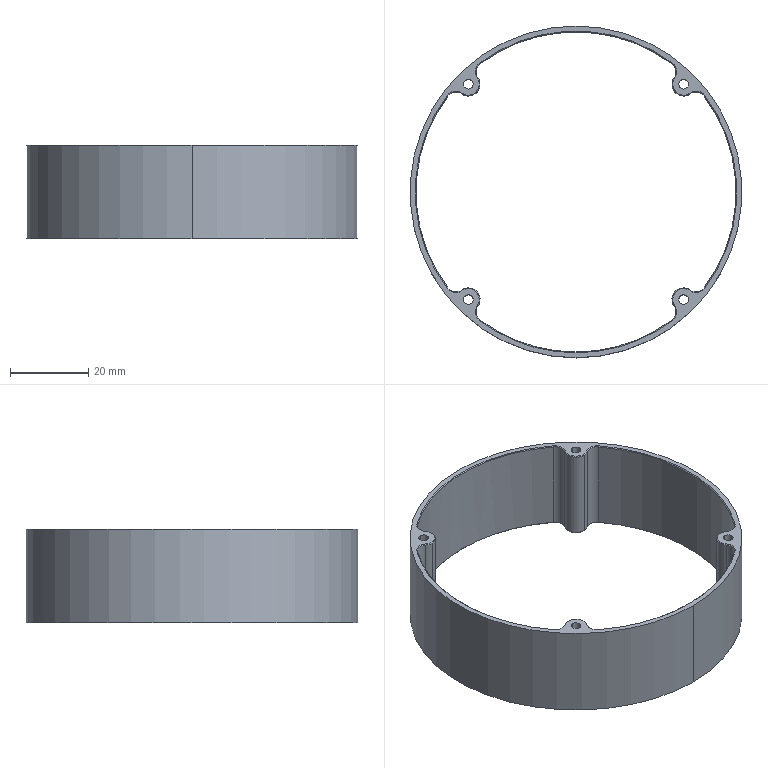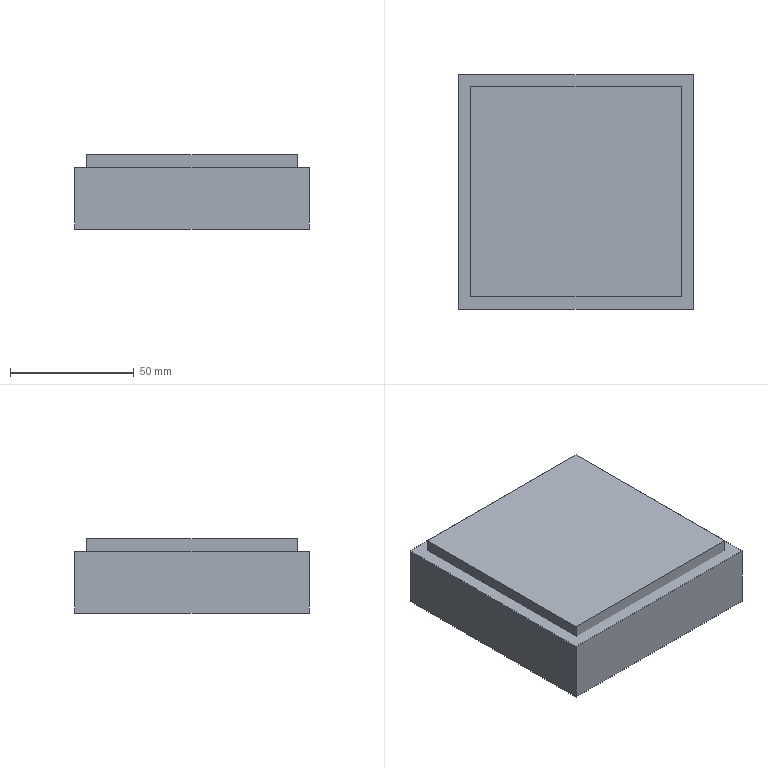CAM job | NX | 3-axis milling, drilling | part box 85 x 85 x 24 mm | stock box 95 x 95 x 30 mm
Tools:
number,name,description,diameter,corner_radius,flute_length,length,flutes
19,D80,Milling Tool-5 Parameters,80.0,0.0,50.0,75.0,2
15,D10,Milling Tool-5 Parameters,10.0,0.0,50.0,75.0,2
14,D10JING,Milling Tool-5 Parameters,10.0,0.0,50.0,75.0,2
1,D6A45,Milling Tool-5 Parameters,6.0,0.0,50.0,75.0,2
2,2.5ZT,Drilling Tool,2.5,0.0,35.0,50.0,2
11,D4,Milling Tool-5 Parameters,4.0,0.0,50.0,75.0,2
Operations:
program,operation,operation_type,tool,method,geometry_group,spindle_rpm,surface_speed,feed_per_tooth,feed_cut,feed_plunge,cut_length_mm,path_length_mm,cut_time_min,machine_time_min
1,FLOOR_WALL,VolumeBased25DMillingOperation,D80,METHOD,A,6500.0,1633.0,0.1154,1500.0,100.0,424.997,478.997,0.2833,0.2887
1,ADAPTIVE_MILLING,CavityMilling,D10,METHOD,A,9500.0,298.0,0.1579,3000.0,1000.0,5438.387,5540.387,1.815,1.825
1,ZLEVEL_PROFILE_COPY_1_COPY_COPY_1,ZLevelMilling,D10JING,METHOD,A,9500.0,298.0,0.0632,1200.0,1000.0,611.882,803.312,0.5112,0.5303
1,PLANAR_MILL_COPY_COPY_COPY_COPY_COPY_COPY_1,PlanarMilling,D6A45,METHOD,A,9500.0,179.0,0.0658,1250.0,100.0,277.785,336.785,0.2222,0.2281
2,FLOOR_WALL_COPY,VolumeBased25DMillingOperation,D80,METHOD,B,6500.0,1633.0,0.1154,1500.0,100.0,2405.982,2964.968,1.604,1.66
2,DRILLING,Operation,D6A45,METHOD,B,5000.0,94.0,0.035,350.0,0.0,18.4,271.508,0.0526,0.0779
2,PLANAR_MILL_COPY_COPY_COPY_COPY_COPY_COPY_1_COPY,PlanarMilling,D6A45,METHOD,B,9500.0,179.0,0.0658,1250.0,100.0,277.785,336.785,0.2222,0.2281
2,PLANAR_MILL_COPY_COPY_COPY_COPY_COPY_COPY_1_COPY_COPY,PlanarMilling,D6A45,METHOD,B,9500.0,179.0,0.0658,1250.0,800.0,275.972,332.972,0.2226,0.2283
2,DRILLING_COPY,Operation,2.5ZT,METHOD,B,2000.0,15.0,0.025,100.0,0.0,117.004,468.716,1.17,1.205
2,PLANAR_MILL,PlanarMilling,D10,METHOD,B,9500.0,0.0,0.0,2200.0,1000.0,39806.758,41679.281,19.002,19.189
2,PLANAR_MILL_COPY,PlanarMilling,D4,METHOD,B,7000.0,87.0,0.0714,1000.0,1000.0,5280.972,8231.098,5.281,5.576
2,刀补,ZLevelMilling,D10JING,METHOD,B,9500.0,298.0,0.0632,1200.0,1000.0,492.804,681.098,0.4119,0.4307